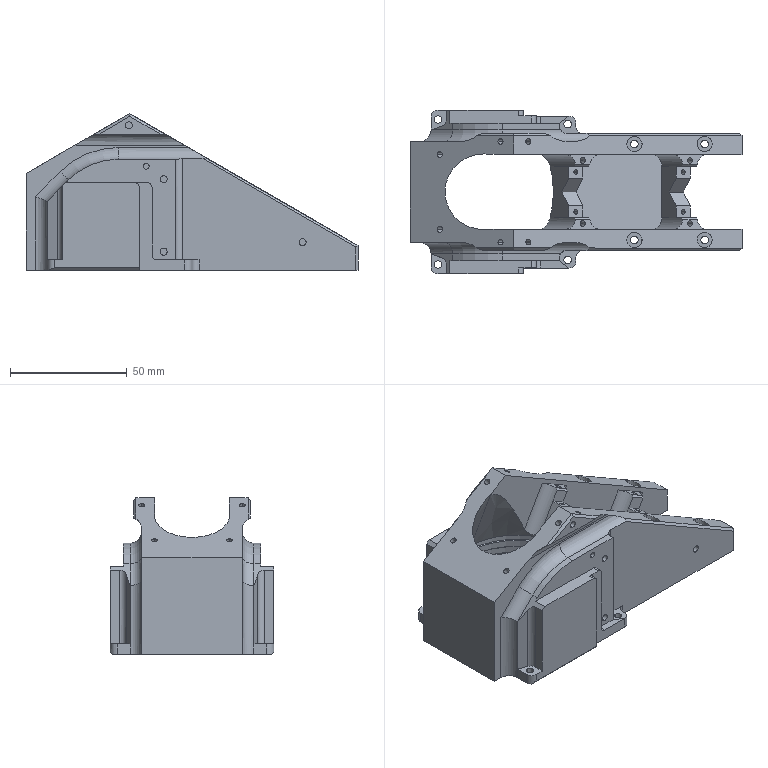NC program | NX | posted with a generic post | part box 142 x 70 x 67 mm
Lines 6452 to 7379 of 58889:
(PLANAR_MILL_COPY_COPY_COPY_COPY_2_COPY_1_COPY_COPY , TOOL : D6R0)
N12824 T20 M6
N12826 G54
N12828 G17 G0 G90 X-68.864 Y30.857 S3000 M3
N12830 G43 Z30. H20
N12832 G94 G1 Z-33. F5000.
N12834 G41 X-68.492 Y30.522 F500. D20
N12836 X-67.608 Y29.78
N12838 G3 X-63.668 Y29.085 R4.
N12840 G1 X-58.5 Y30.966
N12842 Y35.966
N12844 G3 X-60.5 Y39.431 R4.
N12846 G1 X-61.5 Y40.008
N12848 G40
N12850 X-61.941 Y40.243
N12852 G0 Z1.
N12854 X-68.864 Y30.857
N12856 G1 Z-33. F5000.
N12858 G41 X-68.492 Y30.522 F500.
N12860 X-67.608 Y29.78
N12862 G3 X-63.668 Y29.085 R4.
N12864 G1 X-58.5 Y30.966
N12866 Y35.966
N12868 G3 X-60.5 Y39.431 R4.
N12870 G1 X-61.5 Y40.008
N12872 G40
N12874 X-61.941 Y40.243
N12876 G0 Z1.
N12878 X-68.864 Y30.857
N12880 G1 Z-33. F5000.
N12882 G41 X-68.492 Y30.522 F500.
N12884 X-67.608 Y29.78
N12886 G3 X-63.668 Y29.085 R4.
N12888 G1 X-58.5 Y30.966
N12890 Y35.966
N12892 G3 X-60.5 Y39.431 R4.
N12894 G1 X-61.5 Y40.008
N12896 G40
N12898 X-61.941 Y40.243
N12900 G0 Z1.
N12902 X-68.864 Y30.857
N12904 G1 Z-33. F5000.
N12906 G41 X-68.492 Y30.522 F500.
N12908 X-67.608 Y29.78
N12910 G3 X-63.668 Y29.085 R4.
N12912 G1 X-58.5 Y30.966
N12914 Y35.966
N12916 G3 X-60.5 Y39.431 R4.
N12918 G1 X-61.5 Y40.008
N12920 G40
N12922 X-61.941 Y40.243
N12924 G0 Z1.
N12926 X-68.864 Y30.857
N12928 G1 Z-33. F5000.
N12930 G41 X-68.492 Y30.522 F500.
N12932 X-67.608 Y29.78
N12934 G3 X-63.668 Y29.085 R4.
N12936 G1 X-58.5 Y30.966
N12938 Y35.966
N12940 G3 X-60.5 Y39.431 R4.
N12942 G1 X-61.5 Y40.008
N12944 G40
N12946 X-61.941 Y40.243
N12948 G0 Z1.
N12950 X-68.864 Y30.857
N12952 G1 Z-62.5 F5000.
N12954 G41 X-68.492 Y30.522 F500.
N12956 X-67.608 Y29.78
N12958 G3 X-63.668 Y29.085 R4.
N12960 G1 X-58.5 Y30.966
N12962 Y35.966
N12964 G3 X-60.5 Y39.431 R4.
N12966 G1 X-61.5 Y40.008
N12968 G40
N12970 X-61.941 Y40.243
N12972 G0 Z-32.
N12974 X-68.864 Y30.857
N12976 G1 Z-62.5 F5000.
N12978 G41 X-68.492 Y30.522 F500.
N12980 X-67.608 Y29.78
N12982 G3 X-63.668 Y29.085 R4.
N12984 G1 X-58.5 Y30.966
N12986 Y35.966
N12988 G3 X-60.5 Y39.431 R4.
N12990 G1 X-61.5 Y40.008
N12992 G40
N12994 X-61.941 Y40.243
N12996 G0 Z-32.
N12998 X-68.864 Y30.857
N13000 G1 Z-62.5 F5000.
N13002 G41 X-68.492 Y30.522 F500.
N13004 X-67.608 Y29.78
N13006 G3 X-63.668 Y29.085 R4.
N13008 G1 X-58.5 Y30.966
N13010 Y35.966
N13012 G3 X-60.5 Y39.431 R4.
N13014 G1 X-61.5 Y40.008
N13016 G40
N13018 X-61.941 Y40.243
N13020 G0 Z-32.
N13022 X-68.864 Y30.857
N13024 G1 Z-62.5 F5000.
N13026 G41 X-68.492 Y30.522 F500.
N13028 X-67.608 Y29.78
N13030 G3 X-63.668 Y29.085 R4.
N13032 G1 X-58.5 Y30.966
N13034 Y35.966
N13036 G3 X-60.5 Y39.431 R4.
N13038 G1 X-61.5 Y40.008
N13040 G40
N13042 X-61.941 Y40.243
N13044 G0 Z-32.
N13046 X-68.864 Y30.857
N13048 G1 Z-62.5 F5000.
N13050 G41 X-68.492 Y30.522 F500.
N13052 X-67.608 Y29.78
N13054 G3 X-63.668 Y29.085 R4.
N13056 G1 X-58.5 Y30.966
N13058 Y35.966
N13060 G3 X-60.5 Y39.431 R4.
N13062 G1 X-61.5 Y40.008
N13064 G40
N13066 X-61.941 Y40.243
N13068 G0 Z30.
N13070 X-0.659 Y35.276
N13072 G1 Z-33. F5000.
N13074 G41 X-1.1 Y35.041 F500.
N13076 X-2.1 Y34.464
N13078 G3 X-4.1 Y31. R4.
N13080 G1 Y28.
N13082 X7.
N13084 G3 X10.464 Y30. R4.
N13086 G1 X11.041 Y31.
N13088 G40
N13090 X11.276 Y31.441
N13092 G0 Z1.
N13094 X-0.659 Y35.276
N13096 G1 Z-33. F5000.
N13098 G41 X-1.1 Y35.041 F500.
N13100 X-2.1 Y34.464
N13102 G3 X-4.1 Y31. R4.
N13104 G1 Y28.
N13106 X7.
N13108 G3 X10.464 Y30. R4.
N13110 G1 X11.041 Y31.
N13112 G40
N13114 X11.276 Y31.441
N13116 G0 Z1.
N13118 X-0.659 Y35.276
N13120 G1 Z-33. F5000.
N13122 G41 X-1.1 Y35.041 F500.
N13124 X-2.1 Y34.464
N13126 G3 X-4.1 Y31. R4.
N13128 G1 Y28.
N13130 X7.
N13132 G3 X10.464 Y30. R4.
N13134 G1 X11.041 Y31.
N13136 G40
N13138 X11.276 Y31.441
N13140 G0 Z1.
N13142 X-0.659 Y35.276
N13144 G1 Z-33. F5000.
N13146 G41 X-1.1 Y35.041 F500.
N13148 X-2.1 Y34.464
N13150 G3 X-4.1 Y31. R4.
N13152 G1 Y28.
N13154 X7.
N13156 G3 X10.464 Y30. R4.
N13158 G1 X11.041 Y31.
N13160 G40
N13162 X11.276 Y31.441
N13164 G0 Z1.
N13166 X-0.659 Y35.276
N13168 G1 Z-33. F5000.
N13170 G41 X-1.1 Y35.041 F500.
N13172 X-2.1 Y34.464
N13174 G3 X-4.1 Y31. R4.
N13176 G1 Y28.
N13178 X7.
N13180 G3 X10.464 Y30. R4.
N13182 G1 X11.041 Y31.
N13184 G40
N13186 X11.276 Y31.441
N13188 G0 Z1.
N13190 X-0.659 Y35.276
N13192 G1 Z-62.5 F5000.
N13194 G41 X-1.1 Y35.041 F500.
N13196 X-2.1 Y34.464
N13198 G3 X-4.1 Y31. R4.
N13200 G1 Y28.
N13202 X7.
N13204 G3 X10.464 Y30. R4.
N13206 G1 X11.041 Y31.
N13208 G40
N13210 X11.276 Y31.441
N13212 G0 Z-32.
N13214 X-0.659 Y35.276
N13216 G1 Z-62.5 F5000.
N13218 G41 X-1.1 Y35.041 F500.
N13220 X-2.1 Y34.464
N13222 G3 X-4.1 Y31. R4.
N13224 G1 Y28.
N13226 X7.
N13228 G3 X10.464 Y30. R4.
N13230 G1 X11.041 Y31.
N13232 G40
N13234 X11.276 Y31.441
N13236 G0 Z-32.
N13238 X-0.659 Y35.276
N13240 G1 Z-62.5 F5000.
N13242 G41 X-1.1 Y35.041 F500.
N13244 X-2.1 Y34.464
N13246 G3 X-4.1 Y31. R4.
N13248 G1 Y28.
N13250 X7.
N13252 G3 X10.464 Y30. R4.
N13254 G1 X11.041 Y31.
N13256 G40
N13258 X11.276 Y31.441
N13260 G0 Z-32.
N13262 X-0.659 Y35.276
N13264 G1 Z-62.5 F5000.
N13266 G41 X-1.1 Y35.041 F500.
N13268 X-2.1 Y34.464
N13270 G3 X-4.1 Y31. R4.
N13272 G1 Y28.
N13274 X7.
N13276 G3 X10.464 Y30. R4.
N13278 G1 X11.041 Y31.
N13280 G40
N13282 X11.276 Y31.441
N13284 G0 Z-32.
N13286 X-0.659 Y35.276
N13288 G1 Z-62.5 F5000.
N13290 G41 X-1.1 Y35.041 F500.
N13292 X-2.1 Y34.464
N13294 G3 X-4.1 Y31. R4.
N13296 G1 Y28.
N13298 X7.
N13300 G3 X10.464 Y30. R4.
N13302 G1 X11.041 Y31.
N13304 G40
N13306 X11.276 Y31.441
N13308 G0 Z30.
N13310 Y-31.441
N13312 G1 Z-33. F5000.
N13314 G41 X11.041 Y-31. F500.
N13316 X10.464 Y-30.
N13318 G3 X7. Y-28. R4.
N13320 G1 X-4.1
N13322 Y-31.
N13324 G3 X-2.1 Y-34.464 R4.
N13326 G1 X-1.1 Y-35.041
N13328 G40
N13330 X-0.659 Y-35.276
N13332 G0 Z1.
N13334 X11.276 Y-31.441
N13336 G1 Z-33. F5000.
N13338 G41 X11.041 Y-31. F500.
N13340 X10.464 Y-30.
N13342 G3 X7. Y-28. R4.
N13344 G1 X-4.1
N13346 Y-31.
N13348 G3 X-2.1 Y-34.464 R4.
N13350 G1 X-1.1 Y-35.041
N13352 G40
N13354 X-0.659 Y-35.276
N13356 G0 Z1.
N13358 X11.276 Y-31.441
N13360 G1 Z-33. F5000.
N13362 G41 X11.041 Y-31. F500.
N13364 X10.464 Y-30.
N13366 G3 X7. Y-28. R4.
N13368 G1 X-4.1
N13370 Y-31.
N13372 G3 X-2.1 Y-34.464 R4.
N13374 G1 X-1.1 Y-35.041
N13376 G40
N13378 X-0.659 Y-35.276
N13380 G0 Z1.
N13382 X11.276 Y-31.441
N13384 G1 Z-33. F5000.
N13386 G41 X11.041 Y-31. F500.
N13388 X10.464 Y-30.
N13390 G3 X7. Y-28. R4.
N13392 G1 X-4.1
N13394 Y-31.
N13396 G3 X-2.1 Y-34.464 R4.
N13398 G1 X-1.1 Y-35.041
N13400 G40
N13402 X-0.659 Y-35.276
N13404 G0 Z1.
N13406 X11.276 Y-31.441
N13408 G1 Z-33. F5000.
N13410 G41 X11.041 Y-31. F500.
N13412 X10.464 Y-30.
N13414 G3 X7. Y-28. R4.
N13416 G1 X-4.1
N13418 Y-31.
N13420 G3 X-2.1 Y-34.464 R4.
N13422 G1 X-1.1 Y-35.041
N13424 G40
N13426 X-0.659 Y-35.276
N13428 G0 Z1.
N13430 X11.276 Y-31.441
N13432 G1 Z-62.5 F5000.
N13434 G41 X11.041 Y-31. F500.
N13436 X10.464 Y-30.
N13438 G3 X7. Y-28. R4.
N13440 G1 X-4.1
N13442 Y-31.
N13444 G3 X-2.1 Y-34.464 R4.
N13446 G1 X-1.1 Y-35.041
N13448 G40
N13450 X-0.659 Y-35.276
N13452 G0 Z-32.
N13454 X11.276 Y-31.441
N13456 G1 Z-62.5 F5000.
N13458 G41 X11.041 Y-31. F500.
N13460 X10.464 Y-30.
N13462 G3 X7. Y-28. R4.
N13464 G1 X-4.1
N13466 Y-31.
N13468 G3 X-2.1 Y-34.464 R4.
N13470 G1 X-1.1 Y-35.041
N13472 G40
N13474 X-0.659 Y-35.276
N13476 G0 Z-32.
N13478 X11.276 Y-31.441
N13480 G1 Z-62.5 F5000.
N13482 G41 X11.041 Y-31. F500.
N13484 X10.464 Y-30.
N13486 G3 X7. Y-28. R4.
N13488 G1 X-4.1
N13490 Y-31.
N13492 G3 X-2.1 Y-34.464 R4.
N13494 G1 X-1.1 Y-35.041
N13496 G40
N13498 X-0.659 Y-35.276
N13500 G0 Z-32.
N13502 X11.276 Y-31.441
N13504 G1 Z-62.5 F5000.
N13506 G41 X11.041 Y-31. F500.
N13508 X10.464 Y-30.
N13510 G3 X7. Y-28. R4.
N13512 G1 X-4.1
N13514 Y-31.
N13516 G3 X-2.1 Y-34.464 R4.
N13518 G1 X-1.1 Y-35.041
N13520 G40
N13522 X-0.659 Y-35.276
N13524 G0 Z-32.
N13526 X11.276 Y-31.441
N13528 G1 Z-62.5 F5000.
N13530 G41 X11.041 Y-31. F500.
N13532 X10.464 Y-30.
N13534 G3 X7. Y-28. R4.
N13536 G1 X-4.1
N13538 Y-31.
N13540 G3 X-2.1 Y-34.464 R4.
N13542 G1 X-1.1 Y-35.041
N13544 G40
N13546 X-0.659 Y-35.276
N13548 G0 Z30.
N13550 X-61.941 Y-40.243
N13552 G1 Z-33. F5000.
N13554 G41 X-61.5 Y-40.008 F500.
N13556 X-60.5 Y-39.431
N13558 G3 X-58.5 Y-35.966 R4.
N13560 G1 Y-30.966
N13562 X-63.198 Y-29.256
N13564 G3 X-67.138 Y-29.951 R4.
N13566 G1 X-68.022 Y-30.693
N13568 G40
N13570 X-68.394 Y-31.028
N13572 G0 Z1.
N13574 X-61.941 Y-40.243
N13576 G1 Z-33. F5000.
N13578 G41 X-61.5 Y-40.008 F500.
N13580 X-60.5 Y-39.431
N13582 G3 X-58.5 Y-35.966 R4.
N13584 G1 Y-30.966
N13586 X-63.198 Y-29.256
N13588 G3 X-67.138 Y-29.951 R4.
N13590 G1 X-68.022 Y-30.693
N13592 G40
N13594 X-68.394 Y-31.028
N13596 G0 Z1.
N13598 X-61.941 Y-40.243
N13600 G1 Z-33. F5000.
N13602 G41 X-61.5 Y-40.008 F500.
N13604 X-60.5 Y-39.431
N13606 G3 X-58.5 Y-35.966 R4.
N13608 G1 Y-30.966
N13610 X-63.198 Y-29.256
N13612 G3 X-67.138 Y-29.951 R4.
N13614 G1 X-68.022 Y-30.693
N13616 G40
N13618 X-68.394 Y-31.028
N13620 G0 Z1.
N13622 X-61.941 Y-40.243
N13624 G1 Z-33. F5000.
N13626 G41 X-61.5 Y-40.008 F500.
N13628 X-60.5 Y-39.431
N13630 G3 X-58.5 Y-35.966 R4.
N13632 G1 Y-30.966
N13634 X-63.198 Y-29.256
N13636 G3 X-67.138 Y-29.951 R4.
N13638 G1 X-68.022 Y-30.693
N13640 G40
N13642 X-68.394 Y-31.028
N13644 G0 Z1.
N13646 X-61.941 Y-40.243
N13648 G1 Z-33. F5000.
N13650 G41 X-61.5 Y-40.008 F500.
N13652 X-60.5 Y-39.431
N13654 G3 X-58.5 Y-35.966 R4.
N13656 G1 Y-30.966
N13658 X-63.198 Y-29.256
N13660 G3 X-67.138 Y-29.951 R4.
N13662 G1 X-68.022 Y-30.693
N13664 G40
N13666 X-68.394 Y-31.028
N13668 G0 Z1.
N13670 X-61.941 Y-40.243
N13672 G1 Z-62.5 F5000.
N13674 G41 X-61.5 Y-40.008 F500.
N13676 X-60.5 Y-39.431
N13678 G3 X-58.5 Y-35.966 R4.
N13680 G1 Y-30.966
N13682 X-63.198 Y-29.256
N13684 G3 X-67.138 Y-29.951 R4.
N13686 G1 X-68.022 Y-30.693
N13688 G40
N13690 X-68.394 Y-31.028
N13692 G0 Z-32.
N13694 X-61.941 Y-40.243
N13696 G1 Z-62.5 F5000.
N13698 G41 X-61.5 Y-40.008 F500.
N13700 X-60.5 Y-39.431
N13702 G3 X-58.5 Y-35.966 R4.
N13704 G1 Y-30.966
N13706 X-63.198 Y-29.256
N13708 G3 X-67.138 Y-29.951 R4.
N13710 G1 X-68.022 Y-30.693
N13712 G40
N13714 X-68.394 Y-31.028
N13716 G0 Z-32.
N13718 X-61.941 Y-40.243
N13720 G1 Z-62.5 F5000.
N13722 G41 X-61.5 Y-40.008 F500.
N13724 X-60.5 Y-39.431
N13726 G3 X-58.5 Y-35.966 R4.
N13728 G1 Y-30.966
N13730 X-63.198 Y-29.256
N13732 G3 X-67.138 Y-29.951 R4.
N13734 G1 X-68.022 Y-30.693
N13736 G40
N13738 X-68.394 Y-31.028
N13740 G0 Z-32.
N13742 X-61.941 Y-40.243
N13744 G1 Z-62.5 F5000.
N13746 G41 X-61.5 Y-40.008 F500.
N13748 X-60.5 Y-39.431
N13750 G3 X-58.5 Y-35.966 R4.
N13752 G1 Y-30.966
N13754 X-63.198 Y-29.256
N13756 G3 X-67.138 Y-29.951 R4.
N13758 G1 X-68.022 Y-30.693
N13760 G40
N13762 X-68.394 Y-31.028
N13764 G0 Z-32.
N13766 X-61.941 Y-40.243
N13768 G1 Z-62.5 F5000.
N13770 G41 X-61.5 Y-40.008 F500.
N13772 X-60.5 Y-39.431
N13774 G3 X-58.5 Y-35.966 R4.
N13776 G1 Y-30.966
N13778 X-63.198 Y-29.256
N13780 G3 X-67.138 Y-29.951 R4.
N13782 G1 X-68.022 Y-30.693
N13784 G40
N13786 X-68.394 Y-31.028
N13788 G0 Z30.
N13790 M5
(DRILLING , TOOL : DK-D12)
N13792 T05 M6
N13794 G54
N13796 G17 G0 G90 X45. Y20.5 S1800 M3
N13798 G43 Z30. H5
N13800 G94 G81 G99 Z-3. F200. R1.5
N13802 G0 Z20.
N13804 G81 Y-20.5 Z-3. R1.5
N13806 G0 Z20.
N13808 G81 X-63.661 Y-16.5 Z-3. R1.5
N13810 G0 Z20.
N13812 G81 Y16.5 Z-3. R1.5
N13814 G0 Z20.
N13816 G80
N13818 G0 X-63.661 Y16.5 Z30.
(DRILLING_COPY , TOOL : DK-D12)
N13820 X-53.661
N13822 G81 Z-3.9 F200. R1.5
N13824 G0 Z20.
N13826 G81 X31.339 Z-3.9 R1.5
N13828 G0 Z20.
N13830 G80
N13832 G0 X31.339 Y16.5 Z30.
(DRILLING_COPY_2 , TOOL : DK-D12)
N13834 X25. Y20.5
N13836 G81 Z-4. F200. R1.5
N13838 G0 Z20.
N13840 G81 X55. Z-4. R1.5
N13842 G0 Z20.
N13844 G81 Y-20.5 Z-4. R1.5
N13846 G0 Z20.
N13848 G81 X25. Z-4. R1.5
N13850 G0 Z20.
N13852 G80
N13854 G0 X25. Y-20.5 Z30.
(PLANAR_MILL_COPY_COPY_COPY_COPY_COPY_COPY , TOOL : DK-D12)
N13856 X-30.826 Y8.5 S4000
N13858 G1 Z-2. F5000.
N13860 G41 Y12.5 F1000. D5
N13862 X-41.347
N13864 G3 X-44.218 Y11.769 R6.
N13866 X-44.218 Y-11.769 R13.402
N13868 X-41.347 Y-12.5 R6.
N13870 G1 X-20.31
N13872 G3 X-14.541 Y-8.149 R6.
N13874 X-14.534 Y8.144 R29.684
N13876 X-20.304 Y12.5 R6.
N13878 G1 X-30.826
N13880 G40
N13882 Y8.5
N13884 G0 Z30.
(PLANAR_MILL_COPY_COPY_COPY_COPY_COPY_COPY_COPY , TOOL : DK-D12)
N13886 X75.5 Y11.983
N13888 G1 Z-2. F5000.
N13890 G41 X75. Y12. F1000.
N13892 X71.
N13894 X61.
N13896 G3 X55. Y6. R6.
N13898 G1 Y-6.
N13900 G3 X61. Y-12. R6.
N13902 G1 X71.
N13904 X75.
N13906 G40
N13908 X75.5 Y-11.983
N13910 G0 Z30.
(PLANAR_MILL_COPY_COPY_1_COPY_2 , TOOL : DK-D12)
N13912 Z30.35 S5500
N13914 X78.149 Y4.965
N13916 G1 Z-0.8 F5000.
N13918 G41 X77.15 Y5. F1000.
N13920 G3 X72.15 Y0. R5.
N13922 G1 Y-24.
N13924 G2 X71.813 Y-24.813 R1.15
N13926 G1 X70.813 Y-25.813
N13928 G2 X70. Y-26.15 R1.15
N13930 G1 X3.
N13932 G3 X1.15 Y-28. R1.85
N13934 G1 Y-29.5
N13936 G2 X-2.921 Y-33.649 R4.15
N13938 G1 X-22.427 Y-36.15
N13940 X-59.
N13942 G2 X-63.15 Y-32. R4.15
N13944 G1 Y-26.5
N13946 G3 X-67. Y-22.65 R3.85
N13948 G1 X-71.
N13950 G2 X-72.15 Y-21.5 R1.15
N13952 G1 Y21.5
N13954 G2 X-71. Y22.65 R1.15
N13956 G1 X-67.
N13958 G3 X-63.15 Y26.5 R3.85
N13960 G1 Y32.
N13962 G2 X-59. Y36.15 R4.15
N13964 G1 X-22.427
N13966 X-2.921 Y33.649
N13968 G2 X1.15 Y29.5 R4.15
N13970 G1 Y28.
N13972 G3 X3. Y26.15 R1.85
N13974 G1 X70.
N13976 G2 X70.813 Y25.813 R1.15
N13978 G1 X71.813 Y24.813
N13980 G2 X72.15 Y24. R1.15
N13982 G1 Y0.
N13984 G3 X77.15 Y-5. R5.
N13986 G40
N13988 G1 X78.149 Y-4.965
N13990 G0 Z30.35
N13992 M5
(DRILLING_COPY_3 , TOOL : DK-D5)
N13994 T06 M6
N13996 G54
N13998 G17 G0 G90 X-59. Y-31. S1500 M3
N14000 G43 Z30. H6
N14002 G94 G81 G99 Z-64.1 F100. R-61.
N14004 G0 Z17.5
N14006 G81 X-3.6 Y-29. Z-64.1 R-61.
N14008 G0 Z17.5
N14010 G81 Y29. Z-64.1 R-61.
N14012 G0 Z17.5
N14014 G81 X-59. Y31. Z-64.1 R-61.
N14016 G0 Z17.5
N14018 G80
N14020 G0 X-59. Y31. Z30.
N14022 M5
(DRILLING_COPY_1 , TOOL : D05钻头)
N14024 T07 M6
N14026 G54
N14028 G17 G0 G90 X45. Y20.5 S2000 M3
N14030 G43 Z30. H7
N14032 G94 G83 G99 Z-17. F200. Q5. R1.5
N14034 G0 Z20.
N14036 G83 Y-20.5 Z-17. Q5. R1.5
N14038 G0 Z20.
N14040 G83 X-63.661 Y-16.5 Z-17. Q5. R1.5
N14042 G0 Z20.
N14044 G83 Y16.5 Z-17. Q5. R1.5
N14046 G0 Z20.
N14048 G80
N14050 G0 X-63.661 Y16.5 Z30.
(DRILLING_COPY_1_COPY , TOOL : D05钻头)
N14052 X31.339
N14054 G83 Z-10. F200. Q5. R1.5
N14056 G0 Z20.
N14058 G83 X-53.661 Z-10. Q5. R1.5
N14060 G0 Z20.
N14062 G80
N14064 G0 X-53.661 Y16.5 Z30.
N14066 M5
(DRILLING_COPY_1_COPY_1 , TOOL : D6.5钻头)
N14068 T08 M6
N14070 G54
N14072 G17 G0 G90 X25. Y20.5 S2000 M3
N14074 G43 Z30. H8
N14076 G94 G83 G99 Z-62. F200. Q3. R1.5
N14078 G0 Z20.
N14080 G83 X55. Z-62. Q3. R1.5
N14082 G0 Z20.
N14084 G83 Y-20.5 Z-62. Q3. R1.5
N14086 G0 Z20.
N14088 G83 X25. Z-62. Q3. R1.5
N14090 G0 Z20.
N14092 G80
N14094 G0 X25. Y-20.5 Z30.
N14096 M5
(DRILLING_COPY_1_COPY_1_COPY_1 , TOOL : D6.5R0)
N14098 T10 M6
N14100 G54
N14102 G17 G0 G90 X25. Y20.5 S1200 M3
N14104 G43 Z30. H10
N14106 G94 G83 G99 Z-61. F150. Q5. R1.5
N14108 G0 Z20.
N14110 G83 X55. Z-61. Q5. R1.5
N14112 G0 Z20.
N14114 G83 Y-20.5 Z-61. Q5. R1.5
N14116 G0 Z20.
N14118 G83 X25. Z-61. Q5. R1.5
N14120 G0 Z20.
N14122 G80
N14124 G0 X25. Y-20.5 Z30.
N14126 M5
(HOLE_MILLING , TOOL : D4R0)
N14128 T11 M6
N14130 G54
N14132 G17 G0 G90 X-53.661 Y16.5 S5500 M3
N14134 G43 Z30. H11
N14136 G94 G1 Z0.3 F5000.
N14138 G3 X-52.711 Y15.55 R0.95 F1200.
N14140 X-51.761 Y16.5 R0.95
N14142 X-51.761 Y16.5 Z-0.2 I-1.9 J0.
N14144 X-51.761 Y16.5 Z-0.7 I-1.9 J0.
N14146 X-51.761 Y16.5 Z-1.2 I-1.9 J0.
N14148 X-51.761 Y16.5 Z-1.7 I-1.9 J0.
N14150 X-51.761 Y16.5 Z-2.2 I-1.9 J0.
N14152 X-51.761 Y16.5 Z-2.7 I-1.9 J0.
N14154 X-51.761 Y16.5 Z-3.2 I-1.9 J0.
N14156 X-51.761 Y16.5 Z-3.7 I-1.9 J0.
N14158 X-51.761 Y16.5 Z-4.2 I-1.9 J0.
N14160 X-51.761 Y16.5 Z-4.7 I-1.9 J0.
N14162 X-51.761 Y16.5 Z-5.2 I-1.9 J0.
N14164 X-51.761 Y16.5 Z-5.7 I-1.9 J0.
N14166 X-51.761 Y16.5 Z-6.2 I-1.9 J0.
N14168 X-51.761 Y16.5 Z-6.7 I-1.9 J0.
N14170 X-51.761 Y16.5 Z-7.2 I-1.9 J0.
N14172 X-51.761 Y16.5 Z-7.7 I-1.9 J0.
N14174 X-51.761 Y16.5 Z-8.2 I-1.9 J0.
N14176 X-55.198 Y15.383 Z-8.5 R-1.9
N14178 X-52.544 Y14.963 R1.9
N14180 X-55.198 Y15.383 R-1.9
N14182 X-53.871 Y15.173 R0.95
N14184 X-53.661 Y16.5 R0.95
N14186 G0 Z30.
N14188 X31.339
N14190 G1 Z0.3 F5000.
N14192 G3 X32.289 Y15.55 R0.95 F1200.
N14194 X33.239 Y16.5 R0.95
N14196 X33.239 Y16.5 Z-0.2 I-1.9 J0.
N14198 X33.239 Y16.5 Z-0.7 I-1.9 J0.
N14200 X33.239 Y16.5 Z-1.2 I-1.9 J0.
N14202 X33.239 Y16.5 Z-1.7 I-1.9 J0.
N14204 X33.239 Y16.5 Z-2.2 I-1.9 J0.
N14206 X33.239 Y16.5 Z-2.7 I-1.9 J0.
N14208 X33.239 Y16.5 Z-3.2 I-1.9 J0.
N14210 X33.239 Y16.5 Z-3.7 I-1.9 J0.
N14212 X33.239 Y16.5 Z-4.2 I-1.9 J0.
N14214 X33.239 Y16.5 Z-4.7 I-1.9 J0.
N14216 X33.239 Y16.5 Z-5.2 I-1.9 J0.
N14218 X33.239 Y16.5 Z-5.7 I-1.9 J0.
N14220 X33.239 Y16.5 Z-6.2 I-1.9 J0.
N14222 X33.239 Y16.5 Z-6.7 I-1.9 J0.
N14224 X33.239 Y16.5 Z-7.2 I-1.9 J0.
N14226 X33.239 Y16.5 Z-7.7 I-1.9 J0.
N14228 X33.239 Y16.5 Z-8.2 I-1.9 J0.
N14230 X29.802 Y15.383 Z-8.5 R-1.9
N14232 X32.456 Y14.963 R1.9
N14234 X29.802 Y15.383 R-1.9
N14236 X31.129 Y15.173 R0.95
N14238 X31.339 Y16.5 R0.95
N14240 G0 Z30.
(PLANAR_MILL , TOOL : D4R0)
N14242 X31.809 Y16.035
N14244 G1 Z-8. F5000.
N14246 G41 X32.809 Y16. F400. D11
N14248 G3 X33.309 Y16.5 R0.5
N14250 X31.339 Y18.47 R1.97
N14252 X33.309 Y16.5 R-1.97
N14254 X32.809 Y17. R0.5
N14256 G40
N14258 G1 X31.809 Y16.965
N14260 X31.819 Y16.035
N14262 G41 X32.819 Y16.
N14264 G3 X33.319 Y16.5 R0.5
N14266 X31.339 Y18.48 R1.98
N14268 X33.319 Y16.5 R-1.98
N14270 X32.819 Y17. R0.5
N14272 G40
N14274 G1 X31.819 Y16.965
N14276 G0 Z30.
N14278 X-53.191 Y16.035
N14280 G1 Z-8. F5000.
N14282 G41 X-52.191 Y16. F400.
N14284 G3 X-51.691 Y16.5 R0.5
N14286 X-53.661 Y18.47 R1.97
N14288 X-51.691 Y16.5 R-1.97
N14290 X-52.191 Y17. R0.5
N14292 G40
N14294 G1 X-53.191 Y16.965
N14296 X-53.181 Y16.035
N14298 G41 X-52.181 Y16.
N14300 G3 X-51.681 Y16.5 R0.5
N14302 X-53.661 Y18.48 R1.98
N14304 X-51.681 Y16.5 R-1.98
N14306 X-52.181 Y17. R0.5
N14308 G40
N14310 G1 X-53.181 Y16.965
N14312 G0 Z30.
N14314 M5
(PLANAR_MILL_COPY_COPY_1 , TOOL : DJ-D3)
N14316 T12 M6
N14318 G54
N14320 G17 G0 G90 X75.149 Y1.965 S5500 M3
N14322 G43 Z30.35 H12
N14324 G94 G1 Z-0.8 F5000.
N14326 G41 X74.15 Y2. F1000. D12
N14328 G3 X72.15 Y0. R2.
N14330 G1 Y-24.
N14332 G2 X71.813 Y-24.813 R1.15
N14334 G1 X70.813 Y-25.813
N14336 G2 X70. Y-26.15 R1.15
N14338 G1 X3.
N14340 G3 X1.15 Y-28. R1.85
N14342 G1 Y-29.5
N14344 G2 X-2.921 Y-33.649 R4.15
N14346 G1 X-22.427 Y-36.15
N14348 X-59.
N14350 G2 X-63.15 Y-32. R4.15
N14352 G1 Y-26.5
N14354 G3 X-67. Y-22.65 R3.85
N14356 G1 X-71.
N14358 G2 X-72.15 Y-21.5 R1.15
N14360 G1 Y21.5
N14362 G2 X-71. Y22.65 R1.15
N14364 G1 X-67.
N14366 G3 X-63.15 Y26.5 R3.85
N14368 G1 Y32.
N14370 G2 X-59. Y36.15 R4.15
N14372 G1 X-22.427
N14374 X-2.921 Y33.649
N14376 G2 X1.15 Y29.5 R4.15
N14378 G1 Y28.
N14380 G3 X3. Y26.15 R1.85
N14382 G1 X70.
N14384 G2 X70.813 Y25.813 R1.15
N14386 G1 X71.813 Y24.813
N14388 G2 X72.15 Y24. R1.15
N14390 G1 Y0.
N14392 G3 X74.15 Y-2. R2.
N14394 G40
N14396 G1 X75.149 Y-1.965
N14398 G0 Z30.35
(PLANAR_MILL_COPY_COPY_1_COPY_1 , TOOL : DJ-D3)
N14400 X-3.301 Y34.865
N14402 Z30.
N14404 G1 Z-0.8 F5000.
N14406 G41 X-4.3 Y34.9 F1000.
N14408 G3 X-6.3 Y32.9 R2.
N14410 G1 Y28.
N14412 G3 X-4.1 Y25.8 R2.2
N14414 G1 X8.
N14416 G3 X10. Y27.8 R2.
N14418 G40
N14420 G1 X9.965 Y28.799
N14422 G0 Z30.
N14424 Y-28.799
N14426 G1 Z-0.8 F5000.
N14428 G41 X10. Y-27.8 F1000.
N14430 G3 X8. Y-25.8 R2.
N14432 G1 X-4.1
N14434 G3 X-6.3 Y-28. R2.2
N14436 G1 Y-32.9
N14438 G3 X-4.3 Y-34.9 R2.
N14440 G40
N14442 G1 X-3.301 Y-34.865
N14444 G0 Z30.
(PLANAR_MILL_COPY_COPY_1_COPY_1_COPY , TOOL : DJ-D3)
N14446 X-56.335 Y-37.999
N14448 G1 Z-0.8 F5000.
N14450 G41 X-56.3 Y-37. F1000.
N14452 Y-35.
N14454 Y-30.966
N14456 G3 X-57.748 Y-28.899 R2.2
N14458 G1 X-62.274 Y-27.252
N14460 X-64.153 Y-26.568
N14462 G40
N14464 X-65.104 Y-26.259
N14466 G0 Z30.
N14468 Y26.259
N14470 G1 Z-0.8 F5000.
N14472 G41 X-64.153 Y26.568 F1000.
N14474 X-62.274 Y27.252
N14476 X-57.748 Y28.899
N14478 G3 X-56.3 Y30.966 R2.2
N14480 G1 Y35.
N14482 Y37.
N14484 G40
N14486 X-56.335 Y37.999
N14488 G0 Z30.
N14490 M5
(FACE_MILLING_COPY , TOOL : D80)
N14492 T01 M6
N14494 G54
N14496 G17 G0 G90 X176.661 Y16. S3500 M3
N14498 G43 Z105. H1
N14500 G94 G1 Z73.013 F5000.
N14502 X164.661 F1500.
N14504 X-57.339
N14506 X-69.339
N14508 G0 Z85.
N14510 X176.661
N14512 G1 Z71.025 F5000.
N14514 X164.661 F1500.
N14516 X-57.339
N14518 X-69.339
N14520 G0 Z85.
N14522 X176.661
N14524 G1 Z69.038 F5000.
N14526 X164.661 F1500.
N14528 X-57.339
N14530 X-69.339
N14532 G0 Z85.
N14534 X176.661
N14536 G1 Z67.05 F5000.
N14538 X164.661 F1500.
N14540 X-57.339
N14542 X-69.339
N14544 G0 Z105.
N14546 M5
(DRILLING_COPY_2_COPY_COPY , TOOL : U钻-D21)
N14548 T14 M6
N14550 G54
N14552 G17 G0 G90 X17.661 Y16.5 S2000 M3
N14554 G43 Z97. H14
N14556 G94 G83 G99 Z32. F100. Q2. R68.5
N14558 G0 Z87.
N14560 G80
N14562 G0 X17.661 Y16.5 Z97.
N14564 M5